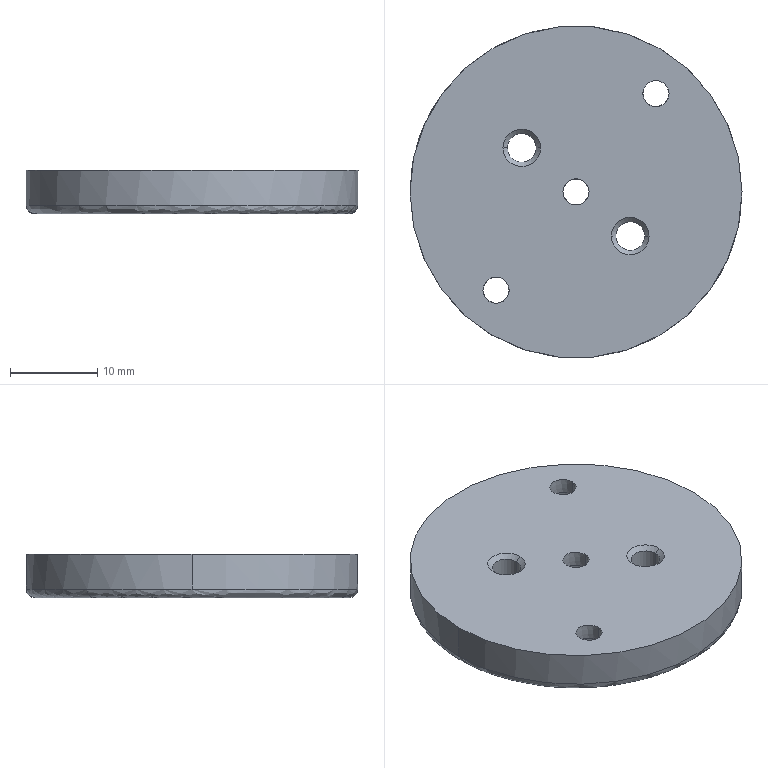Part | SolidWorks | features BaseBody 1 | 1 solid | 33 faces | box 38 x 38 x 5 mm | volume 5246 mm3 | cone 14 | cylinder 12 | plane 5 | spline 2 | commonest cylinder face diameters 6 x6 3.3 x4 38 x2
STEP:
#1=CARTESIAN_POINT('',(479.235,-109.572,230.545));
#2=VERTEX_POINT('',#1);
#3=CARTESIAN_POINT('',(451.305,-86.858,230.545));
#4=VERTEX_POINT('',#3);
#5=CARTESIAN_POINT('',(479.235,-109.572,230.545));
#6=CARTESIAN_POINT('',(501.949,-81.641,230.545));
#7=CARTESIAN_POINT('',(474.019,-58.928,230.545));
#8=CARTESIAN_POINT('',(451.305,-86.858,230.545));
#9=(BOUNDED_CURVE()B_SPLINE_CURVE(3,(#5,#6,#7,#8),.UNSPECIFIED.,.F.,.T.)B_SPLINE_CURVE_WITH_KNOTS((4,4),(0.,1.),.UNSPECIFIED.)CURVE()GEOMETRIC_REPRESENTATION_ITEM()RATIONAL_B_SPLINE_CURVE((1.,0.3333,0.3333,1.))REPRESENTATION_ITEM(''));
#10=EDGE_CURVE('',#2,#4,#9,.T.);
#11=ORIENTED_EDGE('',*,*,#10,.T.);
#12=CARTESIAN_POINT('',(450.529,-86.227,231.545));
#13=VERTEX_POINT('',#12);
#14=CARTESIAN_POINT('',(451.305,-86.858,231.545));
#15=DIRECTION('',(0.6309,0.7758,-0.000000012));
#16=DIRECTION('',(-0.7758,0.6309,0.000000021));
#17=AXIS2_PLACEMENT_3D('',#14,#15,#16);
#18=CIRCLE('',#17,1.);
#19=EDGE_CURVE('',#4,#13,#18,.T.);
#20=ORIENTED_EDGE('',*,*,#19,.T.);
#21=CARTESIAN_POINT('',(484.27,-98.215,231.545));
#22=VERTEX_POINT('',#21);
#23=CARTESIAN_POINT('',(465.27,-98.215,231.545));
#24=DIRECTION('',(0.000000024,-0.000000004,1.));
#25=DIRECTION('',(-1.,0.,0.000000024));
#26=AXIS2_PLACEMENT_3D('',#23,#24,#25);
#27=CIRCLE('',#26,19.);
#28=EDGE_CURVE('',#22,#13,#27,.T.);
#29=ORIENTED_EDGE('',*,*,#28,.F.);
#30=CARTESIAN_POINT('',(480.011,-110.203,231.545));
#31=VERTEX_POINT('',#30);
#32=CARTESIAN_POINT('',(465.27,-98.215,231.545));
#33=DIRECTION('',(0.000000024,-0.000000004,1.));
#34=DIRECTION('',(-1.,0.,0.000000024));
#35=AXIS2_PLACEMENT_3D('',#32,#33,#34);
#36=CIRCLE('',#35,19.);
#37=EDGE_CURVE('',#31,#22,#36,.T.);
#38=ORIENTED_EDGE('',*,*,#37,.F.);
#39=CARTESIAN_POINT('',(479.235,-109.572,231.545));
#40=DIRECTION('',(-0.6309,-0.7758,0.000000012));
#41=DIRECTION('',(0.7758,-0.6309,-0.000000021));
#42=AXIS2_PLACEMENT_3D('',#39,#40,#41);
#43=CIRCLE('',#42,1.);
#44=EDGE_CURVE('',#2,#31,#43,.T.);
#45=ORIENTED_EDGE('',*,*,#44,.F.);
#46=EDGE_LOOP('',(#11,#20,#29,#38,#45));
#47=FACE_OUTER_BOUND('',#46,.T.);
#48=CARTESIAN_POINT('',(451.305,-86.858,230.545));
#49=CARTESIAN_POINT('',(474.019,-58.928,230.545));
#50=CARTESIAN_POINT('',(501.949,-81.641,230.545));
#51=CARTESIAN_POINT('',(479.235,-109.572,230.545));
#52=CARTESIAN_POINT('',(450.851,-86.489,230.545));
#53=CARTESIAN_POINT('',(474.303,-57.649,230.545));
#54=CARTESIAN_POINT('',(503.142,-81.102,230.545));
#55=CARTESIAN_POINT('',(479.69,-109.941,230.545));
#56=CARTESIAN_POINT('',(450.529,-86.227,230.959));
#57=CARTESIAN_POINT('',(474.505,-56.745,230.959));
#58=CARTESIAN_POINT('',(503.987,-80.721,230.959));
#59=CARTESIAN_POINT('',(480.011,-110.203,230.959));
#60=CARTESIAN_POINT('',(450.529,-86.227,231.545));
#61=CARTESIAN_POINT('',(474.505,-56.745,231.545));
#62=CARTESIAN_POINT('',(503.987,-80.721,231.545));
#63=CARTESIAN_POINT('',(480.011,-110.203,231.545));
#64=(BOUNDED_SURFACE()B_SPLINE_SURFACE(3,3,((#48,#49,#50,#51),(#52,#53,#54,#55),(#56,#57,#58,#59),(#60,#61,#62,#63)),.UNSPECIFIED.,.F.,.F.,.F.)B_SPLINE_SURFACE_WITH_KNOTS((4,4),(4,4),(0.,1.),(0.,1.),.UNSPECIFIED.)GEOMETRIC_REPRESENTATION_ITEM()RATIONAL_B_SPLINE_SURFACE(((1.,0.3333,0.3333,1.),(0.8047,0.2682,0.2682,0.8047),(0.8047,0.2682,0.2682,0.8047),(1.,0.3333,0.3333,1.)))REPRESENTATION_ITEM('')SURFACE());
#65=ADVANCED_FACE('',(#47),#64,.T.);
#66=CARTESIAN_POINT('',(457.414,-93.168,235.045));
#67=VERTEX_POINT('',#66);
#68=CARTESIAN_POINT('',(460.714,-93.168,235.045));
#69=VERTEX_POINT('',#68);
#70=CARTESIAN_POINT('',(459.064,-93.168,235.045));
#71=DIRECTION('',(0.000000024,-0.000000004,1.));
#72=DIRECTION('',(-0.7758,0.6309,0.000000021));
#73=AXIS2_PLACEMENT_3D('',#70,#71,#72);
#74=CIRCLE('',#73,1.65);
#75=EDGE_CURVE('',#67,#69,#74,.T.);
#76=ORIENTED_EDGE('',*,*,#75,.F.);
#77=CARTESIAN_POINT('',(456.914,-93.168,235.545));
#78=VERTEX_POINT('',#77);
#79=CARTESIAN_POINT('',(456.914,-93.168,235.545));
#80=DIRECTION('',(-0.7071,-0.000000003,0.7071));
#81=VECTOR('',#80,1000.);
#82=LINE('',#79,#81);
#83=EDGE_CURVE('',#67,#78,#82,.T.);
#84=ORIENTED_EDGE('',*,*,#83,.T.);
#85=CARTESIAN_POINT('',(461.214,-93.168,235.545));
#86=VERTEX_POINT('',#85);
#87=CARTESIAN_POINT('',(459.064,-93.168,235.545));
#88=DIRECTION('',(-0.000000024,0.000000004,-1.));
#89=DIRECTION('',(1.,0.,-0.000000024));
#90=AXIS2_PLACEMENT_3D('',#87,#88,#89);
#91=CIRCLE('',#90,2.15);
#92=EDGE_CURVE('',#86,#78,#91,.T.);
#93=ORIENTED_EDGE('',*,*,#92,.F.);
#94=CARTESIAN_POINT('',(461.214,-93.168,235.545));
#95=DIRECTION('',(0.7071,-0.000000003,0.7071));
#96=VECTOR('',#95,1000.);
#97=LINE('',#94,#96);
#98=EDGE_CURVE('',#69,#86,#97,.T.);
#99=ORIENTED_EDGE('',*,*,#98,.F.);
#100=EDGE_LOOP('',(#76,#84,#93,#99));
#101=FACE_OUTER_BOUND('',#100,.T.);
#102=CARTESIAN_POINT('',(459.064,-93.168,235.545));
#103=DIRECTION('',(0.000000024,-0.000000004,1.));
#104=DIRECTION('',(1.,0.,-0.000000024));
#105=AXIS2_PLACEMENT_3D('',#102,#103,#104);
#106=CONICAL_SURFACE('',#105,2.15,0.7854);
#107=ADVANCED_FACE('',(#101),#106,.F.);
#108=CARTESIAN_POINT('',(484.27,-98.215,235.545));
#109=VERTEX_POINT('',#108);
#110=CARTESIAN_POINT('',(446.27,-98.215,235.545));
#111=VERTEX_POINT('',#110);
#112=CARTESIAN_POINT('',(465.27,-98.215,235.545));
#113=DIRECTION('',(0.000000024,-0.000000004,1.));
#114=DIRECTION('',(-1.,0.,0.000000024));
#115=AXIS2_PLACEMENT_3D('',#112,#113,#114);
#116=CIRCLE('',#115,19.);
#117=EDGE_CURVE('',#109,#111,#116,.T.);
#118=ORIENTED_EDGE('',*,*,#117,.F.);
#119=CARTESIAN_POINT('',(484.27,-98.215,230.545));
#120=DIRECTION('',(-0.000000024,0.000000004,-1.));
#121=VECTOR('',#120,1000.);
#122=LINE('',#119,#121);
#123=EDGE_CURVE('',#109,#22,#122,.T.);
#124=ORIENTED_EDGE('',*,*,#123,.T.);
#125=ORIENTED_EDGE('',*,*,#28,.T.);
#126=CARTESIAN_POINT('',(446.27,-98.215,231.545));
#127=VERTEX_POINT('',#126);
#128=CARTESIAN_POINT('',(465.27,-98.215,231.545));
#129=DIRECTION('',(0.000000024,-0.000000004,1.));
#130=DIRECTION('',(-1.,0.,0.000000024));
#131=AXIS2_PLACEMENT_3D('',#128,#129,#130);
#132=CIRCLE('',#131,19.);
#133=EDGE_CURVE('',#13,#127,#132,.T.);
#134=ORIENTED_EDGE('',*,*,#133,.T.);
#135=CARTESIAN_POINT('',(446.27,-98.215,230.545));
#136=DIRECTION('',(-0.000000024,0.000000004,-1.));
#137=VECTOR('',#136,1000.);
#138=LINE('',#135,#137);
#139=EDGE_CURVE('',#111,#127,#138,.T.);
#140=ORIENTED_EDGE('',*,*,#139,.F.);
#141=EDGE_LOOP('',(#118,#124,#125,#134,#140));
#142=FACE_OUTER_BOUND('',#141,.T.);
#143=CARTESIAN_POINT('',(465.27,-98.215,230.545));
#144=DIRECTION('',(-0.000000024,0.000000004,-1.));
#145=DIRECTION('',(-1.,0.,0.000000024));
#146=AXIS2_PLACEMENT_3D('',#143,#144,#145);
#147=CYLINDRICAL_SURFACE('',#146,19.);
#148=ADVANCED_FACE('',(#142),#147,.T.);
#149=CARTESIAN_POINT('',(475.919,-86.965,235.545));
#150=VERTEX_POINT('',#149);
#151=CARTESIAN_POINT('',(472.919,-86.965,235.545));
#152=VERTEX_POINT('',#151);
#153=CARTESIAN_POINT('',(474.419,-86.965,235.545));
#154=DIRECTION('',(-0.000000024,0.000000004,-1.));
#155=DIRECTION('',(-1.,0.,0.000000024));
#156=AXIS2_PLACEMENT_3D('',#153,#154,#155);
#157=CIRCLE('',#156,1.5);
#158=EDGE_CURVE('',#150,#152,#157,.T.);
#159=ORIENTED_EDGE('',*,*,#158,.F.);
#160=CARTESIAN_POINT('',(475.919,-86.965,233.72));
#161=VERTEX_POINT('',#160);
#162=CARTESIAN_POINT('',(475.919,-86.965,233.72));
#163=DIRECTION('',(0.000008194,0.000000004,-1.));
#164=VECTOR('',#163,1000.);
#165=LINE('',#162,#164);
#166=EDGE_CURVE('',#150,#161,#165,.T.);
#167=ORIENTED_EDGE('',*,*,#166,.T.);
#168=CARTESIAN_POINT('',(472.919,-86.965,233.72));
#169=VERTEX_POINT('',#168);
#170=CARTESIAN_POINT('',(474.419,-86.965,233.72));
#171=DIRECTION('',(0.000000024,-0.000000004,1.));
#172=DIRECTION('',(-1.,0.,0.000000024));
#173=AXIS2_PLACEMENT_3D('',#170,#171,#172);
#174=CIRCLE('',#173,1.5);
#175=EDGE_CURVE('',#169,#161,#174,.T.);
#176=ORIENTED_EDGE('',*,*,#175,.F.);
#177=CARTESIAN_POINT('',(472.919,-86.965,233.72));
#178=DIRECTION('',(-0.000008242,0.000000004,-1.));
#179=VECTOR('',#178,1000.);
#180=LINE('',#177,#179);
#181=EDGE_CURVE('',#152,#169,#180,.T.);
#182=ORIENTED_EDGE('',*,*,#181,.F.);
#183=EDGE_LOOP('',(#159,#167,#176,#182));
#184=FACE_OUTER_BOUND('',#183,.T.);
#185=CARTESIAN_POINT('',(474.419,-86.965,233.72));
#186=DIRECTION('',(-0.000000024,0.000000004,-1.));
#187=DIRECTION('',(-1.,0.,0.000000024));
#188=AXIS2_PLACEMENT_3D('',#185,#186,#187);
#189=CONICAL_SURFACE('',#188,1.5,0.000008218);
#190=ADVANCED_FACE('',(#184),#189,.F.);
#191=CARTESIAN_POINT('',(466.77,-98.215,235.545));
#192=VERTEX_POINT('',#191);
#193=CARTESIAN_POINT('',(463.77,-98.215,235.545));
#194=VERTEX_POINT('',#193);
#195=CARTESIAN_POINT('',(465.27,-98.215,235.545));
#196=DIRECTION('',(-0.000000024,0.000000004,-1.));
#197=DIRECTION('',(-1.,0.,0.000000024));
#198=AXIS2_PLACEMENT_3D('',#195,#196,#197);
#199=CIRCLE('',#198,1.5);
#200=EDGE_CURVE('',#192,#194,#199,.T.);
#201=ORIENTED_EDGE('',*,*,#200,.F.);
#202=CARTESIAN_POINT('',(466.77,-98.215,233.72));
#203=VERTEX_POINT('',#202);
#204=CARTESIAN_POINT('',(466.77,-98.215,233.72));
#205=DIRECTION('',(0.000008194,0.000000004,-1.));
#206=VECTOR('',#205,1000.);
#207=LINE('',#204,#206);
#208=EDGE_CURVE('',#192,#203,#207,.T.);
#209=ORIENTED_EDGE('',*,*,#208,.T.);
#210=CARTESIAN_POINT('',(463.77,-98.215,233.72));
#211=VERTEX_POINT('',#210);
#212=CARTESIAN_POINT('',(465.27,-98.215,233.72));
#213=DIRECTION('',(0.000000024,-0.000000004,1.));
#214=DIRECTION('',(-1.,0.,0.000000024));
#215=AXIS2_PLACEMENT_3D('',#212,#213,#214);
#216=CIRCLE('',#215,1.5);
#217=EDGE_CURVE('',#211,#203,#216,.T.);
#218=ORIENTED_EDGE('',*,*,#217,.F.);
#219=CARTESIAN_POINT('',(463.77,-98.215,233.72));
#220=DIRECTION('',(-0.000008242,0.000000004,-1.));
#221=VECTOR('',#220,1000.);
#222=LINE('',#219,#221);
#223=EDGE_CURVE('',#194,#211,#222,.T.);
#224=ORIENTED_EDGE('',*,*,#223,.F.);
#225=EDGE_LOOP('',(#201,#209,#218,#224));
#226=FACE_OUTER_BOUND('',#225,.T.);
#227=CARTESIAN_POINT('',(465.27,-98.215,233.72));
#228=DIRECTION('',(-0.000000024,0.000000004,-1.));
#229=DIRECTION('',(-1.,0.,0.000000024));
#230=AXIS2_PLACEMENT_3D('',#227,#228,#229);
#231=CONICAL_SURFACE('',#230,1.5,0.000008218);
#232=ADVANCED_FACE('',(#226),#231,.F.);
#233=CARTESIAN_POINT('',(457.622,-109.465,235.545));
#234=VERTEX_POINT('',#233);
#235=CARTESIAN_POINT('',(454.622,-109.465,235.545));
#236=VERTEX_POINT('',#235);
#237=CARTESIAN_POINT('',(456.122,-109.465,235.545));
#238=DIRECTION('',(-0.000000024,0.000000004,-1.));
#239=DIRECTION('',(-1.,0.,0.000000024));
#240=AXIS2_PLACEMENT_3D('',#237,#238,#239);
#241=CIRCLE('',#240,1.5);
#242=EDGE_CURVE('',#234,#236,#241,.T.);
#243=ORIENTED_EDGE('',*,*,#242,.F.);
#244=CARTESIAN_POINT('',(457.622,-109.465,233.72));
#245=VERTEX_POINT('',#244);
#246=CARTESIAN_POINT('',(457.622,-109.465,233.72));
#247=DIRECTION('',(0.000008194,0.000000004,-1.));
#248=VECTOR('',#247,1000.);
#249=LINE('',#246,#248);
#250=EDGE_CURVE('',#234,#245,#249,.T.);
#251=ORIENTED_EDGE('',*,*,#250,.T.);
#252=CARTESIAN_POINT('',(454.622,-109.465,233.72));
#253=VERTEX_POINT('',#252);
#254=CARTESIAN_POINT('',(456.122,-109.465,233.72));
#255=DIRECTION('',(0.000000024,-0.000000004,1.));
#256=DIRECTION('',(-1.,0.,0.000000024));
#257=AXIS2_PLACEMENT_3D('',#254,#255,#256);
#258=CIRCLE('',#257,1.5);
#259=EDGE_CURVE('',#253,#245,#258,.T.);
#260=ORIENTED_EDGE('',*,*,#259,.F.);
#261=CARTESIAN_POINT('',(454.622,-109.465,233.72));
#262=DIRECTION('',(-0.000008242,0.000000004,-1.));
#263=VECTOR('',#262,1000.);
#264=LINE('',#261,#263);
#265=EDGE_CURVE('',#236,#253,#264,.T.);
#266=ORIENTED_EDGE('',*,*,#265,.F.);
#267=EDGE_LOOP('',(#243,#251,#260,#266));
#268=FACE_OUTER_BOUND('',#267,.T.);
#269=CARTESIAN_POINT('',(456.122,-109.465,233.72));
#270=DIRECTION('',(-0.000000024,0.000000004,-1.));
#271=DIRECTION('',(-1.,0.,0.000000024));
#272=AXIS2_PLACEMENT_3D('',#269,#270,#271);
#273=CONICAL_SURFACE('',#272,1.5,0.000008218);
#274=ADVANCED_FACE('',(#268),#273,.F.);
#275=CARTESIAN_POINT('',(469.827,-103.262,235.045));
#276=VERTEX_POINT('',#275);
#277=CARTESIAN_POINT('',(473.127,-103.262,235.045));
#278=VERTEX_POINT('',#277);
#279=CARTESIAN_POINT('',(471.477,-103.262,235.045));
#280=DIRECTION('',(0.000000024,-0.000000004,1.));
#281=DIRECTION('',(-0.7758,0.6309,0.000000021));
#282=AXIS2_PLACEMENT_3D('',#279,#280,#281);
#283=CIRCLE('',#282,1.65);
#284=EDGE_CURVE('',#276,#278,#283,.T.);
#285=ORIENTED_EDGE('',*,*,#284,.F.);
#286=CARTESIAN_POINT('',(469.327,-103.262,235.545));
#287=VERTEX_POINT('',#286);
#288=CARTESIAN_POINT('',(469.327,-103.262,235.545));
#289=DIRECTION('',(-0.7071,-0.000000003,0.7071));
#290=VECTOR('',#289,1000.);
#291=LINE('',#288,#290);
#292=EDGE_CURVE('',#276,#287,#291,.T.);
#293=ORIENTED_EDGE('',*,*,#292,.T.);
#294=CARTESIAN_POINT('',(473.627,-103.262,235.545));
#295=VERTEX_POINT('',#294);
#296=CARTESIAN_POINT('',(471.477,-103.262,235.545));
#297=DIRECTION('',(-0.000000024,0.000000004,-1.));
#298=DIRECTION('',(1.,0.,-0.000000024));
#299=AXIS2_PLACEMENT_3D('',#296,#297,#298);
#300=CIRCLE('',#299,2.15);
#301=EDGE_CURVE('',#295,#287,#300,.T.);
#302=ORIENTED_EDGE('',*,*,#301,.F.);
#303=CARTESIAN_POINT('',(473.627,-103.262,235.545));
#304=DIRECTION('',(0.7071,-0.000000003,0.7071));
#305=VECTOR('',#304,1000.);
#306=LINE('',#303,#305);
#307=EDGE_CURVE('',#278,#295,#306,.T.);
#308=ORIENTED_EDGE('',*,*,#307,.F.);
#309=EDGE_LOOP('',(#285,#293,#302,#308));
#310=FACE_OUTER_BOUND('',#309,.T.);
#311=CARTESIAN_POINT('',(471.477,-103.262,235.545));
#312=DIRECTION('',(0.000000024,-0.000000004,1.));
#313=DIRECTION('',(1.,0.,-0.000000024));
#314=AXIS2_PLACEMENT_3D('',#311,#312,#313);
#315=CONICAL_SURFACE('',#314,2.15,0.7854);
#316=ADVANCED_FACE('',(#310),#315,.F.);
#317=ORIENTED_EDGE('',*,*,#75,.T.);
#318=CARTESIAN_POINT('',(460.714,-93.168,231.045));
#319=VERTEX_POINT('',#318);
#320=CARTESIAN_POINT('',(460.714,-93.168,233.045));
#321=DIRECTION('',(-0.000000024,0.000000004,-1.));
#322=VECTOR('',#321,1000.);
#323=LINE('',#320,#322);
#324=EDGE_CURVE('',#69,#319,#323,.T.);
#325=ORIENTED_EDGE('',*,*,#324,.T.);
#326=CARTESIAN_POINT('',(457.414,-93.168,231.045));
#327=VERTEX_POINT('',#326);
#328=CARTESIAN_POINT('',(459.064,-93.168,231.045));
#329=DIRECTION('',(0.000000024,-0.000000004,1.));
#330=DIRECTION('',(-1.,0.,0.000000024));
#331=AXIS2_PLACEMENT_3D('',#328,#329,#330);
#332=CIRCLE('',#331,1.65);
#333=EDGE_CURVE('',#327,#319,#332,.T.);
#334=ORIENTED_EDGE('',*,*,#333,.F.);
#335=CARTESIAN_POINT('',(457.414,-93.168,233.045));
#336=DIRECTION('',(-0.000000024,0.000000004,-1.));
#337=VECTOR('',#336,1000.);
#338=LINE('',#335,#337);
#339=EDGE_CURVE('',#67,#327,#338,.T.);
#340=ORIENTED_EDGE('',*,*,#339,.F.);
#341=EDGE_LOOP('',(#317,#325,#334,#340));
#342=FACE_OUTER_BOUND('',#341,.T.);
#343=CARTESIAN_POINT('',(459.064,-93.168,233.045));
#344=DIRECTION('',(-0.000000024,0.000000004,-1.));
#345=DIRECTION('',(-1.,0.,0.000000024));
#346=AXIS2_PLACEMENT_3D('',#343,#344,#345);
#347=CYLINDRICAL_SURFACE('',#346,1.65);
#348=ADVANCED_FACE('',(#342),#347,.F.);
#349=ORIENTED_EDGE('',*,*,#284,.T.);
#350=CARTESIAN_POINT('',(473.127,-103.262,231.045));
#351=VERTEX_POINT('',#350);
#352=CARTESIAN_POINT('',(473.127,-103.262,233.045));
#353=DIRECTION('',(-0.000000024,0.000000004,-1.));
#354=VECTOR('',#353,1000.);
#355=LINE('',#352,#354);
#356=EDGE_CURVE('',#278,#351,#355,.T.);
#357=ORIENTED_EDGE('',*,*,#356,.T.);
#358=CARTESIAN_POINT('',(469.827,-103.262,231.045));
#359=VERTEX_POINT('',#358);
#360=CARTESIAN_POINT('',(471.477,-103.262,231.045));
#361=DIRECTION('',(0.000000024,-0.000000004,1.));
#362=DIRECTION('',(-1.,0.,0.000000024));
#363=AXIS2_PLACEMENT_3D('',#360,#361,#362);
#364=CIRCLE('',#363,1.65);
#365=EDGE_CURVE('',#359,#351,#364,.T.);
#366=ORIENTED_EDGE('',*,*,#365,.F.);
#367=CARTESIAN_POINT('',(469.827,-103.262,233.045));
#368=DIRECTION('',(-0.000000024,0.000000004,-1.));
#369=VECTOR('',#368,1000.);
#370=LINE('',#367,#369);
#371=EDGE_CURVE('',#276,#359,#370,.T.);
#372=ORIENTED_EDGE('',*,*,#371,.F.);
#373=EDGE_LOOP('',(#349,#357,#366,#372));
#374=FACE_OUTER_BOUND('',#373,.T.);
#375=CARTESIAN_POINT('',(471.477,-103.262,233.045));
#376=DIRECTION('',(-0.000000024,0.000000004,-1.));
#377=DIRECTION('',(-1.,0.,0.000000024));
#378=AXIS2_PLACEMENT_3D('',#375,#376,#377);
#379=CYLINDRICAL_SURFACE('',#378,1.65);
#380=ADVANCED_FACE('',(#374),#379,.F.);
#381=ORIENTED_EDGE('',*,*,#333,.T.);
#382=CARTESIAN_POINT('',(461.214,-93.168,230.545));
#383=VERTEX_POINT('',#382);
#384=CARTESIAN_POINT('',(461.214,-93.168,230.545));
#385=DIRECTION('',(0.7071,0.000000003,-0.7071));
#386=VECTOR('',#385,1000.);
#387=LINE('',#384,#386);
#388=EDGE_CURVE('',#319,#383,#387,.T.);
#389=ORIENTED_EDGE('',*,*,#388,.T.);
#390=CARTESIAN_POINT('',(456.914,-93.168,230.545));
#391=VERTEX_POINT('',#390);
#392=CARTESIAN_POINT('',(459.064,-93.168,230.545));
#393=DIRECTION('',(0.000000024,-0.000000004,1.));
#394=DIRECTION('',(-1.,0.,0.000000024));
#395=AXIS2_PLACEMENT_3D('',#392,#393,#394);
#396=CIRCLE('',#395,2.15);
#397=EDGE_CURVE('',#391,#383,#396,.T.);
#398=ORIENTED_EDGE('',*,*,#397,.F.);
#399=CARTESIAN_POINT('',(456.914,-93.168,230.545));
#400=DIRECTION('',(-0.7071,0.000000003,-0.7071));
#401=VECTOR('',#400,1000.);
#402=LINE('',#399,#401);
#403=EDGE_CURVE('',#327,#391,#402,.T.);
#404=ORIENTED_EDGE('',*,*,#403,.F.);
#405=EDGE_LOOP('',(#381,#389,#398,#404));
#406=FACE_OUTER_BOUND('',#405,.T.);
#407=CARTESIAN_POINT('',(459.064,-93.168,230.545));
#408=DIRECTION('',(-0.000000024,0.000000004,-1.));
#409=DIRECTION('',(-1.,0.,0.000000024));
#410=AXIS2_PLACEMENT_3D('',#407,#408,#409);
#411=CONICAL_SURFACE('',#410,2.15,0.7854);
#412=ADVANCED_FACE('',(#406),#411,.F.);
#413=CARTESIAN_POINT('',(471.419,-86.965,233.72));
#414=VERTEX_POINT('',#413);
#415=CARTESIAN_POINT('',(477.419,-86.965,233.72));
#416=VERTEX_POINT('',#415);
#417=CARTESIAN_POINT('',(474.419,-86.965,233.72));
#418=DIRECTION('',(0.000000024,-0.000000004,1.));
#419=DIRECTION('',(-1.,0.,0.000000024));
#420=AXIS2_PLACEMENT_3D('',#417,#418,#419);
#421=CIRCLE('',#420,3.);
#422=EDGE_CURVE('',#414,#416,#421,.T.);
#423=ORIENTED_EDGE('',*,*,#422,.T.);
#424=CARTESIAN_POINT('',(477.419,-86.965,230.545));
#425=VERTEX_POINT('',#424);
#426=CARTESIAN_POINT('',(477.419,-86.965,232.132));
#427=DIRECTION('',(-0.000000024,0.000000004,-1.));
#428=VECTOR('',#427,1000.);
#429=LINE('',#426,#428);
#430=EDGE_CURVE('',#416,#425,#429,.T.);
#431=ORIENTED_EDGE('',*,*,#430,.T.);
#432=CARTESIAN_POINT('',(471.419,-86.965,230.545));
#433=VERTEX_POINT('',#432);
#434=CARTESIAN_POINT('',(474.419,-86.965,230.545));
#435=DIRECTION('',(-0.000000024,0.000000004,-1.));
#436=DIRECTION('',(-1.,0.,0.000000024));
#437=AXIS2_PLACEMENT_3D('',#434,#435,#436);
#438=CIRCLE('',#437,3.);
#439=EDGE_CURVE('',#425,#433,#438,.T.);
#440=ORIENTED_EDGE('',*,*,#439,.T.);
#441=CARTESIAN_POINT('',(471.419,-86.965,232.132));
#442=DIRECTION('',(-0.000000024,0.000000004,-1.));
#443=VECTOR('',#442,1000.);
#444=LINE('',#441,#443);
#445=EDGE_CURVE('',#414,#433,#444,.T.);
#446=ORIENTED_EDGE('',*,*,#445,.F.);
#447=EDGE_LOOP('',(#423,#431,#440,#446));
#448=FACE_OUTER_BOUND('',#447,.T.);
#449=CARTESIAN_POINT('',(474.419,-86.965,232.132));
#450=DIRECTION('',(-0.000000024,0.000000004,-1.));
#451=DIRECTION('',(-1.,0.,0.000000024));
#452=AXIS2_PLACEMENT_3D('',#449,#450,#451);
#453=CYLINDRICAL_SURFACE('',#452,3.);
#454=ADVANCED_FACE('',(#448),#453,.F.);
#455=CARTESIAN_POINT('',(462.27,-98.215,233.72));
#456=VERTEX_POINT('',#455);
#457=CARTESIAN_POINT('',(468.27,-98.215,233.72));
#458=VERTEX_POINT('',#457);
#459=CARTESIAN_POINT('',(465.27,-98.215,233.72));
#460=DIRECTION('',(0.000000024,-0.000000004,1.));
#461=DIRECTION('',(-1.,0.,0.000000024));
#462=AXIS2_PLACEMENT_3D('',#459,#460,#461);
#463=CIRCLE('',#462,3.);
#464=EDGE_CURVE('',#456,#458,#463,.T.);
#465=ORIENTED_EDGE('',*,*,#464,.T.);
#466=CARTESIAN_POINT('',(468.27,-98.215,230.545));
#467=VERTEX_POINT('',#466);
#468=CARTESIAN_POINT('',(468.27,-98.215,232.132));
#469=DIRECTION('',(-0.000000024,0.000000004,-1.));
#470=VECTOR('',#469,1000.);
#471=LINE('',#468,#470);
#472=EDGE_CURVE('',#458,#467,#471,.T.);
#473=ORIENTED_EDGE('',*,*,#472,.T.);
#474=CARTESIAN_POINT('',(462.27,-98.215,230.545));
#475=VERTEX_POINT('',#474);
#476=CARTESIAN_POINT('',(465.27,-98.215,230.545));
#477=DIRECTION('',(-0.000000024,0.000000004,-1.));
#478=DIRECTION('',(-1.,0.,0.000000024));
#479=AXIS2_PLACEMENT_3D('',#476,#477,#478);
#480=CIRCLE('',#479,3.);
#481=EDGE_CURVE('',#467,#475,#480,.T.);
#482=ORIENTED_EDGE('',*,*,#481,.T.);
#483=CARTESIAN_POINT('',(462.27,-98.215,232.132));
#484=DIRECTION('',(-0.000000024,0.000000004,-1.));
#485=VECTOR('',#484,1000.);
#486=LINE('',#483,#485);
#487=EDGE_CURVE('',#456,#475,#486,.T.);
#488=ORIENTED_EDGE('',*,*,#487,.F.);
#489=EDGE_LOOP('',(#465,#473,#482,#488));
#490=FACE_OUTER_BOUND('',#489,.T.);
#491=CARTESIAN_POINT('',(465.27,-98.215,232.132));
#492=DIRECTION('',(-0.000000024,0.000000004,-1.));
#493=DIRECTION('',(-1.,0.,0.000000024));
#494=AXIS2_PLACEMENT_3D('',#491,#492,#493);
#495=CYLINDRICAL_SURFACE('',#494,3.);
#496=ADVANCED_FACE('',(#490),#495,.F.);
#497=CARTESIAN_POINT('',(453.122,-109.465,233.72));
#498=VERTEX_POINT('',#497);
#499=CARTESIAN_POINT('',(459.122,-109.465,233.72));
#500=VERTEX_POINT('',#499);
#501=CARTESIAN_POINT('',(456.122,-109.465,233.72));
#502=DIRECTION('',(0.000000024,-0.000000004,1.));
#503=DIRECTION('',(-1.,0.,0.000000024));
#504=AXIS2_PLACEMENT_3D('',#501,#502,#503);
#505=CIRCLE('',#504,3.);
#506=EDGE_CURVE('',#498,#500,#505,.T.);
#507=ORIENTED_EDGE('',*,*,#506,.T.);
#508=CARTESIAN_POINT('',(459.122,-109.465,230.545));
#509=VERTEX_POINT('',#508);
#510=CARTESIAN_POINT('',(459.122,-109.465,232.132));
#511=DIRECTION('',(-0.000000024,0.000000004,-1.));
#512=VECTOR('',#511,1000.);
#513=LINE('',#510,#512);
#514=EDGE_CURVE('',#500,#509,#513,.T.);
#515=ORIENTED_EDGE('',*,*,#514,.T.);
#516=CARTESIAN_POINT('',(453.122,-109.465,230.545));
#517=VERTEX_POINT('',#516);
#518=CARTESIAN_POINT('',(456.122,-109.465,230.545));
#519=DIRECTION('',(-0.000000024,0.000000004,-1.));
#520=DIRECTION('',(-1.,0.,0.000000024));
#521=AXIS2_PLACEMENT_3D('',#518,#519,#520);
#522=CIRCLE('',#521,3.);
#523=EDGE_CURVE('',#509,#517,#522,.T.);
#524=ORIENTED_EDGE('',*,*,#523,.T.);
#525=CARTESIAN_POINT('',(453.122,-109.465,232.132));
#526=DIRECTION('',(-0.000000024,0.000000004,-1.));
#527=VECTOR('',#526,1000.);
#528=LINE('',#525,#527);
#529=EDGE_CURVE('',#498,#517,#528,.T.);
#530=ORIENTED_EDGE('',*,*,#529,.F.);
#531=EDGE_LOOP('',(#507,#515,#524,#530));
#532=FACE_OUTER_BOUND('',#531,.T.);
#533=CARTESIAN_POINT('',(456.122,-109.465,232.132));
#534=DIRECTION('',(-0.000000024,0.000000004,-1.));
#535=DIRECTION('',(-1.,0.,0.000000024));
#536=AXIS2_PLACEMENT_3D('',#533,#534,#535);
#537=CYLINDRICAL_SURFACE('',#536,3.);
#538=ADVANCED_FACE('',(#532),#537,.F.);
#539=ORIENTED_EDGE('',*,*,#365,.T.);
#540=CARTESIAN_POINT('',(473.627,-103.262,230.545));
#541=VERTEX_POINT('',#540);
#542=CARTESIAN_POINT('',(473.627,-103.262,230.545));
#543=DIRECTION('',(0.7071,0.000000003,-0.7071));
#544=VECTOR('',#543,1000.);
#545=LINE('',#542,#544);
#546=EDGE_CURVE('',#351,#541,#545,.T.);
#547=ORIENTED_EDGE('',*,*,#546,.T.);
#548=CARTESIAN_POINT('',(469.327,-103.262,230.545));
#549=VERTEX_POINT('',#548);
#550=CARTESIAN_POINT('',(471.477,-103.262,230.545));
#551=DIRECTION('',(-0.000000024,0.000000004,-1.));
#552=DIRECTION('',(-1.,0.,0.000000024));
#553=AXIS2_PLACEMENT_3D('',#550,#551,#552);
#554=CIRCLE('',#553,2.15);
#555=EDGE_CURVE('',#541,#549,#554,.T.);
#556=ORIENTED_EDGE('',*,*,#555,.T.);
#557=CARTESIAN_POINT('',(469.327,-103.262,230.545));
#558=DIRECTION('',(-0.7071,0.000000003,-0.7071));
#559=VECTOR('',#558,1000.);
#560=LINE('',#557,#559);
#561=EDGE_CURVE('',#359,#549,#560,.T.);
#562=ORIENTED_EDGE('',*,*,#561,.F.);
#563=EDGE_LOOP('',(#539,#547,#556,#562));
#564=FACE_OUTER_BOUND('',#563,.T.);
#565=CARTESIAN_POINT('',(471.477,-103.262,230.545));
#566=DIRECTION('',(-0.000000024,0.000000004,-1.));
#567=DIRECTION('',(-1.,0.,0.000000024));
#568=AXIS2_PLACEMENT_3D('',#565,#566,#567);
#569=CONICAL_SURFACE('',#568,2.15,0.7854);
#570=ADVANCED_FACE('',(#564),#569,.F.);
#571=ORIENTED_EDGE('',*,*,#92,.T.);
#572=CARTESIAN_POINT('',(459.064,-93.168,235.545));
#573=DIRECTION('',(-0.000000024,0.000000004,-1.));
#574=DIRECTION('',(1.,0.,-0.000000024));
#575=AXIS2_PLACEMENT_3D('',#572,#573,#574);
#576=CIRCLE('',#575,2.15);
#577=EDGE_CURVE('',#78,#86,#576,.T.);
#578=ORIENTED_EDGE('',*,*,#577,.T.);
#579=EDGE_LOOP('',(#571,#578));
#580=FACE_BOUND('',#579,.T.);
#581=CARTESIAN_POINT('',(465.27,-98.215,235.545));
#582=DIRECTION('',(0.000000024,-0.000000004,1.));
#583=DIRECTION('',(-1.,0.,0.000000024));
#584=AXIS2_PLACEMENT_3D('',#581,#582,#583);
#585=CIRCLE('',#584,19.);
#586=EDGE_CURVE('',#111,#109,#585,.T.);
#587=ORIENTED_EDGE('',*,*,#586,.T.);
#588=ORIENTED_EDGE('',*,*,#117,.T.);
#589=EDGE_LOOP('',(#587,#588));
#590=FACE_OUTER_BOUND('',#589,.T.);
#591=CARTESIAN_POINT('',(474.419,-86.965,235.545));
#592=DIRECTION('',(-0.000000024,0.000000004,-1.));
#593=DIRECTION('',(-1.,0.,0.000000024));
#594=AXIS2_PLACEMENT_3D('',#591,#592,#593);
#595=CIRCLE('',#594,1.5);
#596=EDGE_CURVE('',#152,#150,#595,.T.);
#597=ORIENTED_EDGE('',*,*,#596,.T.);
#598=ORIENTED_EDGE('',*,*,#158,.T.);
#599=EDGE_LOOP('',(#597,#598));
#600=FACE_BOUND('',#599,.T.);
#601=CARTESIAN_POINT('',(465.27,-98.215,235.545));
#602=DIRECTION('',(-0.000000024,0.000000004,-1.));
#603=DIRECTION('',(-1.,0.,0.000000024));
#604=AXIS2_PLACEMENT_3D('',#601,#602,#603);
#605=CIRCLE('',#604,1.5);
#606=EDGE_CURVE('',#194,#192,#605,.T.);
#607=ORIENTED_EDGE('',*,*,#606,.T.);
#608=ORIENTED_EDGE('',*,*,#200,.T.);
#609=EDGE_LOOP('',(#607,#608));
#610=FACE_BOUND('',#609,.T.);
#611=CARTESIAN_POINT('',(456.122,-109.465,235.545));
#612=DIRECTION('',(-0.000000024,0.000000004,-1.));
#613=DIRECTION('',(-1.,0.,0.000000024));
#614=AXIS2_PLACEMENT_3D('',#611,#612,#613);
#615=CIRCLE('',#614,1.5);
#616=EDGE_CURVE('',#236,#234,#615,.T.);
#617=ORIENTED_EDGE('',*,*,#616,.T.);
#618=ORIENTED_EDGE('',*,*,#242,.T.);
#619=EDGE_LOOP('',(#617,#618));
#620=FACE_BOUND('',#619,.T.);
#621=ORIENTED_EDGE('',*,*,#301,.T.);
#622=CARTESIAN_POINT('',(471.477,-103.262,235.545));
#623=DIRECTION('',(-0.000000024,0.000000004,-1.));
#624=DIRECTION('',(1.,0.,-0.000000024));
#625=AXIS2_PLACEMENT_3D('',#622,#623,#624);
#626=CIRCLE('',#625,2.15);
#627=EDGE_CURVE('',#287,#295,#626,.T.);
#628=ORIENTED_EDGE('',*,*,#627,.T.);
#629=EDGE_LOOP('',(#621,#628));
#630=FACE_BOUND('',#629,.T.);
#631=CARTESIAN_POINT('',(465.27,-98.215,235.545));
#632=DIRECTION('',(0.000000024,-0.000000004,1.));
#633=DIRECTION('',(1.,0.,-0.000000024));
#634=AXIS2_PLACEMENT_3D('',#631,#632,#633);
#635=PLANE('',#634);
#636=ADVANCED_FACE('',(#580,#590,#600,#610,#620,#630),#635,.T.);
#637=ORIENTED_EDGE('',*,*,#83,.F.);
#638=CARTESIAN_POINT('',(459.064,-93.168,235.045));
#639=DIRECTION('',(0.000000024,-0.000000004,1.));
#640=DIRECTION('',(-0.7758,0.6309,0.000000021));
#641=AXIS2_PLACEMENT_3D('',#638,#639,#640);
#642=CIRCLE('',#641,1.65);
#643=EDGE_CURVE('',#69,#67,#642,.T.);
#644=ORIENTED_EDGE('',*,*,#643,.F.);
#645=ORIENTED_EDGE('',*,*,#98,.T.);
#646=ORIENTED_EDGE('',*,*,#577,.F.);
#647=EDGE_LOOP('',(#637,#644,#645,#646));
#648=FACE_OUTER_BOUND('',#647,.T.);
#649=CARTESIAN_POINT('',(459.064,-93.168,235.545));
#650=DIRECTION('',(0.000000024,-0.000000004,1.));
#651=DIRECTION('',(1.,0.,-0.000000024));
#652=AXIS2_PLACEMENT_3D('',#649,#650,#651);
#653=CONICAL_SURFACE('',#652,2.15,0.7854);
#654=ADVANCED_FACE('',(#648),#653,.F.);
#655=ORIENTED_EDGE('',*,*,#123,.F.);
#656=ORIENTED_EDGE('',*,*,#586,.F.);
#657=ORIENTED_EDGE('',*,*,#139,.T.);
#658=CARTESIAN_POINT('',(465.27,-98.215,231.545));
#659=DIRECTION('',(0.000000024,-0.000000004,1.));
#660=DIRECTION('',(-1.,0.,0.000000024));
#661=AXIS2_PLACEMENT_3D('',#658,#659,#660);
#662=CIRCLE('',#661,19.);
#663=EDGE_CURVE('',#127,#31,#662,.T.);
#664=ORIENTED_EDGE('',*,*,#663,.T.);
#665=ORIENTED_EDGE('',*,*,#37,.T.);
#666=EDGE_LOOP('',(#655,#656,#657,#664,#665));
#667=FACE_OUTER_BOUND('',#666,.T.);
#668=CARTESIAN_POINT('',(465.27,-98.215,230.545));
#669=DIRECTION('',(-0.000000024,0.000000004,-1.));
#670=DIRECTION('',(-1.,0.,0.000000024));
#671=AXIS2_PLACEMENT_3D('',#668,#669,#670);
#672=CYLINDRICAL_SURFACE('',#671,19.);
#673=ADVANCED_FACE('',(#667),#672,.T.);
#674=ORIENTED_EDGE('',*,*,#166,.F.);
#675=ORIENTED_EDGE('',*,*,#596,.F.);
#676=ORIENTED_EDGE('',*,*,#181,.T.);
#677=CARTESIAN_POINT('',(474.419,-86.965,233.72));
#678=DIRECTION('',(0.000000024,-0.000000004,1.));
#679=DIRECTION('',(-1.,0.,0.000000024));
#680=AXIS2_PLACEMENT_3D('',#677,#678,#679);
#681=CIRCLE('',#680,1.5);
#682=EDGE_CURVE('',#161,#169,#681,.T.);
#683=ORIENTED_EDGE('',*,*,#682,.F.);
#684=EDGE_LOOP('',(#674,#675,#676,#683));
#685=FACE_OUTER_BOUND('',#684,.T.);
#686=CARTESIAN_POINT('',(474.419,-86.965,233.72));
#687=DIRECTION('',(-0.000000024,0.000000004,-1.));
#688=DIRECTION('',(-1.,0.,0.000000024));
#689=AXIS2_PLACEMENT_3D('',#686,#687,#688);
#690=CONICAL_SURFACE('',#689,1.5,0.000008218);
#691=ADVANCED_FACE('',(#685),#690,.F.);
#692=ORIENTED_EDGE('',*,*,#208,.F.);
#693=ORIENTED_EDGE('',*,*,#606,.F.);
#694=ORIENTED_EDGE('',*,*,#223,.T.);
#695=CARTESIAN_POINT('',(465.27,-98.215,233.72));
#696=DIRECTION('',(0.000000024,-0.000000004,1.));
#697=DIRECTION('',(-1.,0.,0.000000024));
#698=AXIS2_PLACEMENT_3D('',#695,#696,#697);
#699=CIRCLE('',#698,1.5);
#700=EDGE_CURVE('',#203,#211,#699,.T.);
#701=ORIENTED_EDGE('',*,*,#700,.F.);
#702=EDGE_LOOP('',(#692,#693,#694,#701));
#703=FACE_OUTER_BOUND('',#702,.T.);
#704=CARTESIAN_POINT('',(465.27,-98.215,233.72));
#705=DIRECTION('',(-0.000000024,0.000000004,-1.));
#706=DIRECTION('',(-1.,0.,0.000000024));
#707=AXIS2_PLACEMENT_3D('',#704,#705,#706);
#708=CONICAL_SURFACE('',#707,1.5,0.000008218);
#709=ADVANCED_FACE('',(#703),#708,.F.);
#710=ORIENTED_EDGE('',*,*,#250,.F.);
#711=ORIENTED_EDGE('',*,*,#616,.F.);
#712=ORIENTED_EDGE('',*,*,#265,.T.);
#713=CARTESIAN_POINT('',(456.122,-109.465,233.72));
#714=DIRECTION('',(0.000000024,-0.000000004,1.));
#715=DIRECTION('',(-1.,0.,0.000000024));
#716=AXIS2_PLACEMENT_3D('',#713,#714,#715);
#717=CIRCLE('',#716,1.5);
#718=EDGE_CURVE('',#245,#253,#717,.T.);
#719=ORIENTED_EDGE('',*,*,#718,.F.);
#720=EDGE_LOOP('',(#710,#711,#712,#719));
#721=FACE_OUTER_BOUND('',#720,.T.);
#722=CARTESIAN_POINT('',(456.122,-109.465,233.72));
#723=DIRECTION('',(-0.000000024,0.000000004,-1.));
#724=DIRECTION('',(-1.,0.,0.000000024));
#725=AXIS2_PLACEMENT_3D('',#722,#723,#724);
#726=CONICAL_SURFACE('',#725,1.5,0.000008218);
#727=ADVANCED_FACE('',(#721),#726,.F.);
#728=ORIENTED_EDGE('',*,*,#292,.F.);
#729=CARTESIAN_POINT('',(471.477,-103.262,235.045));
#730=DIRECTION('',(0.000000024,-0.000000004,1.));
#731=DIRECTION('',(-0.7758,0.6309,0.000000021));
#732=AXIS2_PLACEMENT_3D('',#729,#730,#731);
#733=CIRCLE('',#732,1.65);
#734=EDGE_CURVE('',#278,#276,#733,.T.);
#735=ORIENTED_EDGE('',*,*,#734,.F.);
#736=ORIENTED_EDGE('',*,*,#307,.T.);
#737=ORIENTED_EDGE('',*,*,#627,.F.);
#738=EDGE_LOOP('',(#728,#735,#736,#737));
#739=FACE_OUTER_BOUND('',#738,.T.);
#740=CARTESIAN_POINT('',(471.477,-103.262,235.545));
#741=DIRECTION('',(0.000000024,-0.000000004,1.));
#742=DIRECTION('',(1.,0.,-0.000000024));
#743=AXIS2_PLACEMENT_3D('',#740,#741,#742);
#744=CONICAL_SURFACE('',#743,2.15,0.7854);
#745=ADVANCED_FACE('',(#739),#744,.F.);
#746=ORIENTED_EDGE('',*,*,#324,.F.);
#747=ORIENTED_EDGE('',*,*,#643,.T.);
#748=ORIENTED_EDGE('',*,*,#339,.T.);
#749=CARTESIAN_POINT('',(459.064,-93.168,231.045));
#750=DIRECTION('',(0.000000024,-0.000000004,1.));
#751=DIRECTION('',(-1.,0.,0.000000024));
#752=AXIS2_PLACEMENT_3D('',#749,#750,#751);
#753=CIRCLE('',#752,1.65);
#754=EDGE_CURVE('',#319,#327,#753,.T.);
#755=ORIENTED_EDGE('',*,*,#754,.F.);
#756=EDGE_LOOP('',(#746,#747,#748,#755));
#757=FACE_OUTER_BOUND('',#756,.T.);
#758=CARTESIAN_POINT('',(459.064,-93.168,233.045));
#759=DIRECTION('',(-0.000000024,0.000000004,-1.));
#760=DIRECTION('',(-1.,0.,0.000000024));
#761=AXIS2_PLACEMENT_3D('',#758,#759,#760);
#762=CYLINDRICAL_SURFACE('',#761,1.65);
#763=ADVANCED_FACE('',(#757),#762,.F.);
#764=ORIENTED_EDGE('',*,*,#19,.F.);
#765=CARTESIAN_POINT('',(451.305,-86.858,230.545));
#766=CARTESIAN_POINT('',(428.592,-114.788,230.545));
#767=CARTESIAN_POINT('',(456.522,-137.502,230.545));
#768=CARTESIAN_POINT('',(479.235,-109.572,230.545));
#769=(BOUNDED_CURVE()B_SPLINE_CURVE(3,(#765,#766,#767,#768),.UNSPECIFIED.,.F.,.F.)B_SPLINE_CURVE_WITH_KNOTS((4,4),(0.,1.),.UNSPECIFIED.)CURVE()GEOMETRIC_REPRESENTATION_ITEM()RATIONAL_B_SPLINE_CURVE((1.,0.3333,0.3333,1.))REPRESENTATION_ITEM(''));
#770=EDGE_CURVE('',#4,#2,#769,.T.);
#771=ORIENTED_EDGE('',*,*,#770,.T.);
#772=ORIENTED_EDGE('',*,*,#44,.T.);
#773=ORIENTED_EDGE('',*,*,#663,.F.);
#774=ORIENTED_EDGE('',*,*,#133,.F.);
#775=EDGE_LOOP('',(#764,#771,#772,#773,#774));
#776=FACE_OUTER_BOUND('',#775,.T.);
#777=CARTESIAN_POINT('',(479.235,-109.572,230.545));
#778=CARTESIAN_POINT('',(456.522,-137.502,230.545));
#779=CARTESIAN_POINT('',(428.592,-114.788,230.545));
#780=CARTESIAN_POINT('',(451.305,-86.858,230.545));
#781=CARTESIAN_POINT('',(479.69,-109.941,230.545));
#782=CARTESIAN_POINT('',(456.237,-138.78,230.545));
#783=CARTESIAN_POINT('',(427.398,-115.328,230.545));
#784=CARTESIAN_POINT('',(450.851,-86.489,230.545));
#785=CARTESIAN_POINT('',(480.011,-110.203,230.959));
#786=CARTESIAN_POINT('',(456.036,-139.685,230.959));
#787=CARTESIAN_POINT('',(426.554,-115.709,230.959));
#788=CARTESIAN_POINT('',(450.529,-86.227,230.959));
#789=CARTESIAN_POINT('',(480.011,-110.203,231.545));
#790=CARTESIAN_POINT('',(456.036,-139.685,231.545));
#791=CARTESIAN_POINT('',(426.554,-115.709,231.545));
#792=CARTESIAN_POINT('',(450.529,-86.227,231.545));
#793=(BOUNDED_SURFACE()B_SPLINE_SURFACE(3,3,((#777,#778,#779,#780),(#781,#782,#783,#784),(#785,#786,#787,#788),(#789,#790,#791,#792)),.UNSPECIFIED.,.F.,.F.,.F.)B_SPLINE_SURFACE_WITH_KNOTS((4,4),(4,4),(0.,1.),(0.,1.),.UNSPECIFIED.)GEOMETRIC_REPRESENTATION_ITEM()RATIONAL_B_SPLINE_SURFACE(((1.,0.3333,0.3333,1.),(0.8047,0.2682,0.2682,0.8047),(0.8047,0.2682,0.2682,0.8047),(1.,0.3333,0.3333,1.)))REPRESENTATION_ITEM('')SURFACE());
#794=ADVANCED_FACE('',(#776),#793,.T.);
#795=ORIENTED_EDGE('',*,*,#422,.F.);
#796=CARTESIAN_POINT('',(474.419,-86.965,233.72));
#797=DIRECTION('',(0.000000024,-0.000000004,1.));
#798=DIRECTION('',(-1.,0.,0.000000024));
#799=AXIS2_PLACEMENT_3D('',#796,#797,#798);
#800=CIRCLE('',#799,3.);
#801=EDGE_CURVE('',#416,#414,#800,.T.);
#802=ORIENTED_EDGE('',*,*,#801,.F.);
#803=EDGE_LOOP('',(#795,#802));
#804=FACE_OUTER_BOUND('',#803,.T.);
#805=ORIENTED_EDGE('',*,*,#175,.T.);
#806=ORIENTED_EDGE('',*,*,#682,.T.);
#807=EDGE_LOOP('',(#805,#806));
#808=FACE_BOUND('',#807,.T.);
#809=CARTESIAN_POINT('',(472.999,-88.711,233.72));
#810=DIRECTION('',(0.000000024,-0.000000004,1.));
#811=DIRECTION('',(1.,0.,-0.000000024));
#812=AXIS2_PLACEMENT_3D('',#809,#810,#811);
#813=PLANE('',#812);
#814=ADVANCED_FACE('',(#804,#808),#813,.F.);
#815=ORIENTED_EDGE('',*,*,#464,.F.);
#816=CARTESIAN_POINT('',(465.27,-98.215,233.72));
#817=DIRECTION('',(0.000000024,-0.000000004,1.));
#818=DIRECTION('',(-1.,0.,0.000000024));
#819=AXIS2_PLACEMENT_3D('',#816,#817,#818);
#820=CIRCLE('',#819,3.);
#821=EDGE_CURVE('',#458,#456,#820,.T.);
#822=ORIENTED_EDGE('',*,*,#821,.F.);
#823=EDGE_LOOP('',(#815,#822));
#824=FACE_OUTER_BOUND('',#823,.T.);
#825=ORIENTED_EDGE('',*,*,#217,.T.);
#826=ORIENTED_EDGE('',*,*,#700,.T.);
#827=EDGE_LOOP('',(#825,#826));
#828=FACE_BOUND('',#827,.T.);
#829=CARTESIAN_POINT('',(463.851,-99.961,233.72));
#830=DIRECTION('',(0.000000024,-0.000000004,1.));
#831=DIRECTION('',(1.,0.,-0.000000024));
#832=AXIS2_PLACEMENT_3D('',#829,#830,#831);
#833=PLANE('',#832);
#834=ADVANCED_FACE('',(#824,#828),#833,.F.);
#835=ORIENTED_EDGE('',*,*,#506,.F.);
#836=CARTESIAN_POINT('',(456.122,-109.465,233.72));
#837=DIRECTION('',(0.000000024,-0.000000004,1.));
#838=DIRECTION('',(-1.,0.,0.000000024));
#839=AXIS2_PLACEMENT_3D('',#836,#837,#838);
#840=CIRCLE('',#839,3.);
#841=EDGE_CURVE('',#500,#498,#840,.T.);
#842=ORIENTED_EDGE('',*,*,#841,.F.);
#843=EDGE_LOOP('',(#835,#842));
#844=FACE_OUTER_BOUND('',#843,.T.);
#845=ORIENTED_EDGE('',*,*,#259,.T.);
#846=ORIENTED_EDGE('',*,*,#718,.T.);
#847=EDGE_LOOP('',(#845,#846));
#848=FACE_BOUND('',#847,.T.);
#849=CARTESIAN_POINT('',(454.702,-111.21,233.72));
#850=DIRECTION('',(0.000000024,-0.000000004,1.));
#851=DIRECTION('',(1.,0.,-0.000000024));
#852=AXIS2_PLACEMENT_3D('',#849,#850,#851);
#853=PLANE('',#852);
#854=ADVANCED_FACE('',(#844,#848),#853,.F.);
#855=ORIENTED_EDGE('',*,*,#356,.F.);
#856=ORIENTED_EDGE('',*,*,#734,.T.);
#857=ORIENTED_EDGE('',*,*,#371,.T.);
#858=CARTESIAN_POINT('',(471.477,-103.262,231.045));
#859=DIRECTION('',(0.000000024,-0.000000004,1.));
#860=DIRECTION('',(-1.,0.,0.000000024));
#861=AXIS2_PLACEMENT_3D('',#858,#859,#860);
#862=CIRCLE('',#861,1.65);
#863=EDGE_CURVE('',#351,#359,#862,.T.);
#864=ORIENTED_EDGE('',*,*,#863,.F.);
#865=EDGE_LOOP('',(#855,#856,#857,#864));
#866=FACE_OUTER_BOUND('',#865,.T.);
#867=CARTESIAN_POINT('',(471.477,-103.262,233.045));
#868=DIRECTION('',(-0.000000024,0.000000004,-1.));
#869=DIRECTION('',(-1.,0.,0.000000024));
#870=AXIS2_PLACEMENT_3D('',#867,#868,#869);
#871=CYLINDRICAL_SURFACE('',#870,1.65);
#872=ADVANCED_FACE('',(#866),#871,.F.);
#873=ORIENTED_EDGE('',*,*,#388,.F.);
#874=ORIENTED_EDGE('',*,*,#754,.T.);
#875=ORIENTED_EDGE('',*,*,#403,.T.);
#876=CARTESIAN_POINT('',(459.064,-93.168,230.545));
#877=DIRECTION('',(0.000000024,-0.000000004,1.));
#878=DIRECTION('',(-1.,0.,0.000000024));
#879=AXIS2_PLACEMENT_3D('',#876,#877,#878);
#880=CIRCLE('',#879,2.15);
#881=EDGE_CURVE('',#383,#391,#880,.T.);
#882=ORIENTED_EDGE('',*,*,#881,.F.);
#883=EDGE_LOOP('',(#873,#874,#875,#882));
#884=FACE_OUTER_BOUND('',#883,.T.);
#885=CARTESIAN_POINT('',(459.064,-93.168,230.545));
#886=DIRECTION('',(-0.000000024,0.000000004,-1.));
#887=DIRECTION('',(-1.,0.,0.000000024));
#888=AXIS2_PLACEMENT_3D('',#885,#886,#887);
#889=CONICAL_SURFACE('',#888,2.15,0.7854);
#890=ADVANCED_FACE('',(#884),#889,.F.);
#891=CARTESIAN_POINT('',(471.477,-103.262,230.545));
#892=DIRECTION('',(-0.000000024,0.000000004,-1.));
#893=DIRECTION('',(-1.,0.,0.000000024));
#894=AXIS2_PLACEMENT_3D('',#891,#892,#893);
#895=CIRCLE('',#894,2.15);
#896=EDGE_CURVE('',#549,#541,#895,.T.);
#897=ORIENTED_EDGE('',*,*,#896,.F.);
#898=ORIENTED_EDGE('',*,*,#555,.F.);
#899=EDGE_LOOP('',(#897,#898));
#900=FACE_BOUND('',#899,.T.);
#901=ORIENTED_EDGE('',*,*,#10,.F.);
#902=ORIENTED_EDGE('',*,*,#770,.F.);
#903=EDGE_LOOP('',(#901,#902));
#904=FACE_OUTER_BOUND('',#903,.T.);
#905=CARTESIAN_POINT('',(474.419,-86.965,230.545));
#906=DIRECTION('',(-0.000000024,0.000000004,-1.));
#907=DIRECTION('',(-1.,0.,0.000000024));
#908=AXIS2_PLACEMENT_3D('',#905,#906,#907);
#909=CIRCLE('',#908,3.);
#910=EDGE_CURVE('',#433,#425,#909,.T.);
#911=ORIENTED_EDGE('',*,*,#910,.F.);
#912=ORIENTED_EDGE('',*,*,#439,.F.);
#913=EDGE_LOOP('',(#911,#912));
#914=FACE_BOUND('',#913,.T.);
#915=CARTESIAN_POINT('',(465.27,-98.215,230.545));
#916=DIRECTION('',(-0.000000024,0.000000004,-1.));
#917=DIRECTION('',(-1.,0.,0.000000024));
#918=AXIS2_PLACEMENT_3D('',#915,#916,#917);
#919=CIRCLE('',#918,3.);
#920=EDGE_CURVE('',#475,#467,#919,.T.);
#921=ORIENTED_EDGE('',*,*,#920,.F.);
#922=ORIENTED_EDGE('',*,*,#481,.F.);
#923=EDGE_LOOP('',(#921,#922));
#924=FACE_BOUND('',#923,.T.);
#925=CARTESIAN_POINT('',(456.122,-109.465,230.545));
#926=DIRECTION('',(-0.000000024,0.000000004,-1.));
#927=DIRECTION('',(-1.,0.,0.000000024));
#928=AXIS2_PLACEMENT_3D('',#925,#926,#927);
#929=CIRCLE('',#928,3.);
#930=EDGE_CURVE('',#517,#509,#929,.T.);
#931=ORIENTED_EDGE('',*,*,#930,.F.);
#932=ORIENTED_EDGE('',*,*,#523,.F.);
#933=EDGE_LOOP('',(#931,#932));
#934=FACE_BOUND('',#933,.T.);
#935=ORIENTED_EDGE('',*,*,#397,.T.);
#936=ORIENTED_EDGE('',*,*,#881,.T.);
#937=EDGE_LOOP('',(#935,#936));
#938=FACE_BOUND('',#937,.T.);
#939=CARTESIAN_POINT('',(465.27,-98.215,230.545));
#940=DIRECTION('',(0.000000024,-0.000000004,1.));
#941=DIRECTION('',(1.,0.,-0.000000024));
#942=AXIS2_PLACEMENT_3D('',#939,#940,#941);
#943=PLANE('',#942);
#944=ADVANCED_FACE('',(#900,#904,#914,#924,#934,#938),#943,.F.);
#945=ORIENTED_EDGE('',*,*,#430,.F.);
#946=ORIENTED_EDGE('',*,*,#801,.T.);
#947=ORIENTED_EDGE('',*,*,#445,.T.);
#948=ORIENTED_EDGE('',*,*,#910,.T.);
#949=EDGE_LOOP('',(#945,#946,#947,#948));
#950=FACE_OUTER_BOUND('',#949,.T.);
#951=CARTESIAN_POINT('',(474.419,-86.965,232.132));
#952=DIRECTION('',(-0.000000024,0.000000004,-1.));
#953=DIRECTION('',(-1.,0.,0.000000024));
#954=AXIS2_PLACEMENT_3D('',#951,#952,#953);
#955=CYLINDRICAL_SURFACE('',#954,3.);
#956=ADVANCED_FACE('',(#950),#955,.F.);
#957=ORIENTED_EDGE('',*,*,#472,.F.);
#958=ORIENTED_EDGE('',*,*,#821,.T.);
#959=ORIENTED_EDGE('',*,*,#487,.T.);
#960=ORIENTED_EDGE('',*,*,#920,.T.);
#961=EDGE_LOOP('',(#957,#958,#959,#960));
#962=FACE_OUTER_BOUND('',#961,.T.);
#963=CARTESIAN_POINT('',(465.27,-98.215,232.132));
#964=DIRECTION('',(-0.000000024,0.000000004,-1.));
#965=DIRECTION('',(-1.,0.,0.000000024));
#966=AXIS2_PLACEMENT_3D('',#963,#964,#965);
#967=CYLINDRICAL_SURFACE('',#966,3.);
#968=ADVANCED_FACE('',(#962),#967,.F.);
#969=ORIENTED_EDGE('',*,*,#514,.F.);
#970=ORIENTED_EDGE('',*,*,#841,.T.);
#971=ORIENTED_EDGE('',*,*,#529,.T.);
#972=ORIENTED_EDGE('',*,*,#930,.T.);
#973=EDGE_LOOP('',(#969,#970,#971,#972));
#974=FACE_OUTER_BOUND('',#973,.T.);
#975=CARTESIAN_POINT('',(456.122,-109.465,232.132));
#976=DIRECTION('',(-0.000000024,0.000000004,-1.));
#977=DIRECTION('',(-1.,0.,0.000000024));
#978=AXIS2_PLACEMENT_3D('',#975,#976,#977);
#979=CYLINDRICAL_SURFACE('',#978,3.);
#980=ADVANCED_FACE('',(#974),#979,.F.);
#981=ORIENTED_EDGE('',*,*,#546,.F.);
#982=ORIENTED_EDGE('',*,*,#863,.T.);
#983=ORIENTED_EDGE('',*,*,#561,.T.);
#984=ORIENTED_EDGE('',*,*,#896,.T.);
#985=EDGE_LOOP('',(#981,#982,#983,#984));
#986=FACE_OUTER_BOUND('',#985,.T.);
#987=CARTESIAN_POINT('',(471.477,-103.262,230.545));
#988=DIRECTION('',(-0.000000024,0.000000004,-1.));
#989=DIRECTION('',(-1.,0.,0.000000024));
#990=AXIS2_PLACEMENT_3D('',#987,#988,#989);
#991=CONICAL_SURFACE('',#990,2.15,0.7854);
#992=ADVANCED_FACE('',(#986),#991,.F.);
#993=CLOSED_SHELL('',(#65,#107,#148,#190,#232,#274,#316,#348,#380,#412,#454,#496,#538,#570,#636,#654,#673,#691,#709,#727,#745,#763,#794,#814,#834,#854,#872,#890,#944,#956,#968,#980,#992));
#994=MANIFOLD_SOLID_BREP('',#993);
#995=CARTESIAN_POINT('',(0.,0.,0.));
#996=DIRECTION('',(0.,0.,1.));
#997=DIRECTION('',(1.,0.,0.));
#998=AXIS2_PLACEMENT_3D('',#995,#996,#997);
#999=(LENGTH_UNIT()NAMED_UNIT(*)SI_UNIT(.MILLI.,.METRE.));
#1000=UNCERTAINTY_MEASURE_WITH_UNIT(LENGTH_MEASURE(0.00001),#999,'','');
#1001=(NAMED_UNIT(*)PLANE_ANGLE_UNIT()SI_UNIT($,.RADIAN.));
#1002=(NAMED_UNIT(*)SI_UNIT($,.STERADIAN.)SOLID_ANGLE_UNIT());
#1003=(GEOMETRIC_REPRESENTATION_CONTEXT(3)GLOBAL_UNCERTAINTY_ASSIGNED_CONTEXT((#1000))GLOBAL_UNIT_ASSIGNED_CONTEXT((#999,#1001,#1002))REPRESENTATION_CONTEXT('',''));
#1004=ADVANCED_BREP_SHAPE_REPRESENTATION('',(#994,#998),#1003);